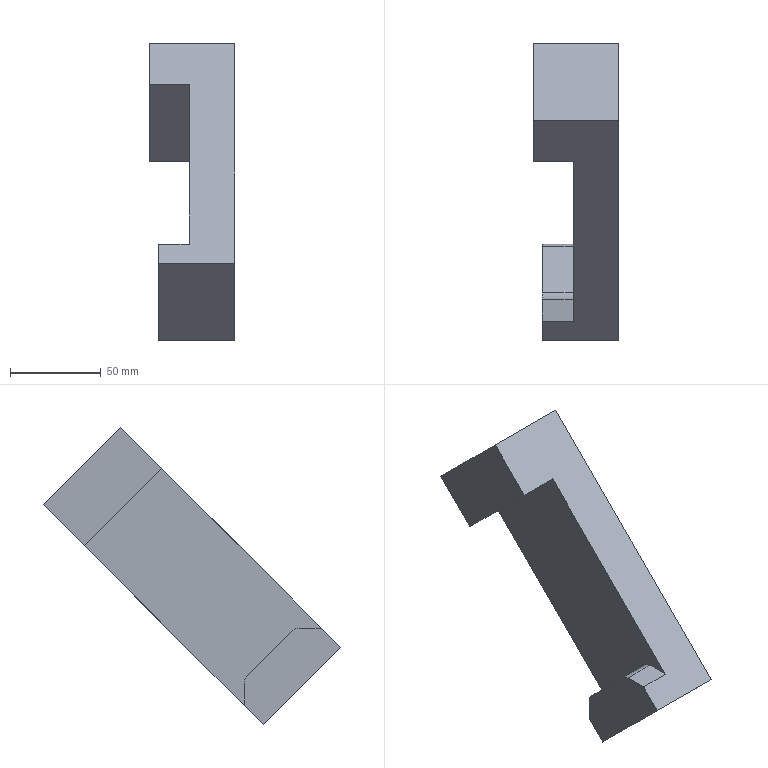Part | NX | features solid 2 | 1 solid | 14 faces | box 47 x 163.342 x 163.342 mm | volume 322522 mm3 | plane 12 | cylinder 2 | commonest cylinder face diameters 10 x2
STEP:
#1=CARTESIAN_POINT('',(757.,887.53,-215.901));
#2=VERTEX_POINT('',#1);
#3=CARTESIAN_POINT('',(757.,975.212,-128.22));
#4=VERTEX_POINT('',#3);
#5=CARTESIAN_POINT('',(757.,937.382,-166.05));
#6=DIRECTION('',(0.,0.7071,0.7071));
#7=VECTOR('',#6,1000.);
#8=LINE('',#5,#7);
#9=EDGE_CURVE('',#2,#4,#8,.T.);
#10=ORIENTED_EDGE('',*,*,#9,.T.);
#11=CARTESIAN_POINT('',(757.,1017.638,-170.646));
#12=VERTEX_POINT('',#11);
#13=CARTESIAN_POINT('',(757.,975.212,-128.22));
#14=DIRECTION('',(0.,0.7071,-0.7071));
#15=VECTOR('',#14,1000.);
#16=LINE('',#13,#15);
#17=EDGE_CURVE('',#4,#12,#16,.T.);
#18=ORIENTED_EDGE('',*,*,#17,.T.);
#19=CARTESIAN_POINT('',(757.,929.957,-258.327));
#20=VERTEX_POINT('',#19);
#21=CARTESIAN_POINT('',(757.,979.808,-208.476));
#22=DIRECTION('',(0.,-0.7071,-0.7071));
#23=VECTOR('',#22,1000.);
#24=LINE('',#21,#23);
#25=EDGE_CURVE('',#12,#20,#24,.T.);
#26=ORIENTED_EDGE('',*,*,#25,.T.);
#27=CARTESIAN_POINT('',(757.,929.957,-246.256));
#28=VERTEX_POINT('',#27);
#29=CARTESIAN_POINT('',(757.,929.957,-258.327));
#30=DIRECTION('',(0.,0.,1.));
#31=VECTOR('',#30,1000.);
#32=LINE('',#29,#31);
#33=EDGE_CURVE('',#28,#20,#32,.F.);
#34=ORIENTED_EDGE('',*,*,#33,.F.);
#35=CARTESIAN_POINT('',(757.,928.492,-242.721));
#36=VERTEX_POINT('',#35);
#37=CARTESIAN_POINT('',(757.,924.957,-246.256));
#38=DIRECTION('',(1.,0.,0.));
#39=DIRECTION('',(0.,-0.9962,-0.08716));
#40=AXIS2_PLACEMENT_3D('',#37,#38,#39);
#41=CIRCLE('',#40,5.);
#42=EDGE_CURVE('',#36,#28,#41,.F.);
#43=ORIENTED_EDGE('',*,*,#42,.F.);
#44=CARTESIAN_POINT('',(757.,903.137,-217.365));
#45=VERTEX_POINT('',#44);
#46=CARTESIAN_POINT('',(757.,894.602,-208.83));
#47=DIRECTION('',(0.,0.7071,-0.7071));
#48=VECTOR('',#47,1000.);
#49=LINE('',#46,#48);
#50=EDGE_CURVE('',#45,#36,#49,.T.);
#51=ORIENTED_EDGE('',*,*,#50,.F.);
#52=CARTESIAN_POINT('',(757.,899.602,-215.901));
#53=VERTEX_POINT('',#52);
#54=CARTESIAN_POINT('',(757.,899.602,-220.901));
#55=DIRECTION('',(1.,0.,0.));
#56=DIRECTION('',(0.,-0.9962,-0.08716));
#57=AXIS2_PLACEMENT_3D('',#54,#55,#56);
#58=CIRCLE('',#57,5.);
#59=EDGE_CURVE('',#53,#45,#58,.F.);
#60=ORIENTED_EDGE('',*,*,#59,.F.);
#61=CARTESIAN_POINT('',(757.,901.673,-215.901));
#62=DIRECTION('',(0.,-1.,0.));
#63=VECTOR('',#62,1000.);
#64=LINE('',#61,#63);
#65=EDGE_CURVE('',#2,#53,#64,.F.);
#66=ORIENTED_EDGE('',*,*,#65,.F.);
#67=EDGE_LOOP('',(#10,#18,#26,#34,#43,#51,#60,#66));
#68=FACE_BOUND('',#67,.T.);
#69=CARTESIAN_POINT('',(757.,958.595,-187.263));
#70=DIRECTION('',(-1.,0.,0.));
#71=DIRECTION('',(0.,-0.7071,-0.7071));
#72=AXIS2_PLACEMENT_3D('',#69,#70,#71);
#73=PLANE('',#72);
#74=ADVANCED_FACE('',(#68),#73,.T.);
#75=CARTESIAN_POINT('',(740.,876.924,-226.508));
#76=VERTEX_POINT('',#75);
#77=CARTESIAN_POINT('',(740.,887.53,-215.901));
#78=VERTEX_POINT('',#77);
#79=CARTESIAN_POINT('',(740.,876.924,-226.508));
#80=DIRECTION('',(0.,0.7071,0.7071));
#81=VECTOR('',#80,1000.);
#82=LINE('',#79,#81);
#83=EDGE_CURVE('',#76,#78,#82,.T.);
#84=ORIENTED_EDGE('',*,*,#83,.F.);
#85=CARTESIAN_POINT('',(782.,876.924,-226.508));
#86=VERTEX_POINT('',#85);
#87=CARTESIAN_POINT('',(782.,876.924,-226.508));
#88=DIRECTION('',(-1.,0.,0.));
#89=VECTOR('',#88,1000.);
#90=LINE('',#87,#89);
#91=EDGE_CURVE('',#86,#76,#90,.T.);
#92=ORIENTED_EDGE('',*,*,#91,.F.);
#93=CARTESIAN_POINT('',(782.,997.839,-105.592));
#94=VERTEX_POINT('',#93);
#95=CARTESIAN_POINT('',(782.,937.382,-166.05));
#96=DIRECTION('',(0.,-0.7071,-0.7071));
#97=VECTOR('',#96,1000.);
#98=LINE('',#95,#97);
#99=EDGE_CURVE('',#94,#86,#98,.T.);
#100=ORIENTED_EDGE('',*,*,#99,.F.);
#101=CARTESIAN_POINT('',(735.,997.839,-105.592));
#102=VERTEX_POINT('',#101);
#103=CARTESIAN_POINT('',(782.,997.839,-105.592));
#104=DIRECTION('',(-1.,0.,0.));
#105=VECTOR('',#104,1000.);
#106=LINE('',#103,#105);
#107=EDGE_CURVE('',#94,#102,#106,.T.);
#108=ORIENTED_EDGE('',*,*,#107,.T.);
#109=CARTESIAN_POINT('',(735.,975.212,-128.22));
#110=VERTEX_POINT('',#109);
#111=CARTESIAN_POINT('',(735.,997.839,-105.592));
#112=DIRECTION('',(0.,-0.7071,-0.7071));
#113=VECTOR('',#112,1000.);
#114=LINE('',#111,#113);
#115=EDGE_CURVE('',#110,#102,#114,.F.);
#116=ORIENTED_EDGE('',*,*,#115,.F.);
#117=CARTESIAN_POINT('',(757.,975.212,-128.22));
#118=DIRECTION('',(1.,0.,0.));
#119=VECTOR('',#118,1000.);
#120=LINE('',#117,#119);
#121=EDGE_CURVE('',#4,#110,#120,.F.);
#122=ORIENTED_EDGE('',*,*,#121,.F.);
#123=ORIENTED_EDGE('',*,*,#9,.F.);
#124=CARTESIAN_POINT('',(782.,887.53,-215.901));
#125=DIRECTION('',(1.,0.,0.));
#126=VECTOR('',#125,1000.);
#127=LINE('',#124,#126);
#128=EDGE_CURVE('',#78,#2,#127,.T.);
#129=ORIENTED_EDGE('',*,*,#128,.F.);
#130=EDGE_LOOP('',(#84,#92,#100,#108,#116,#122,#123,#129));
#131=FACE_BOUND('',#130,.T.);
#132=CARTESIAN_POINT('',(782.,937.382,-166.05));
#133=DIRECTION('',(0.,-0.7071,0.7071));
#134=DIRECTION('',(1.,0.,0.));
#135=AXIS2_PLACEMENT_3D('',#132,#133,#134);
#136=PLANE('',#135);
#137=ADVANCED_FACE('',(#131),#136,.T.);
#138=ORIENTED_EDGE('',*,*,#107,.F.);
#139=CARTESIAN_POINT('',(782.,1040.266,-148.019));
#140=VERTEX_POINT('',#139);
#141=CARTESIAN_POINT('',(782.,1019.052,-126.806));
#142=DIRECTION('',(0.,-0.7071,0.7071));
#143=VECTOR('',#142,1000.);
#144=LINE('',#141,#143);
#145=EDGE_CURVE('',#140,#94,#144,.T.);
#146=ORIENTED_EDGE('',*,*,#145,.F.);
#147=CARTESIAN_POINT('',(735.,1040.266,-148.019));
#148=VERTEX_POINT('',#147);
#149=CARTESIAN_POINT('',(782.,1040.266,-148.019));
#150=DIRECTION('',(-1.,0.,0.));
#151=VECTOR('',#150,1000.);
#152=LINE('',#149,#151);
#153=EDGE_CURVE('',#140,#148,#152,.T.);
#154=ORIENTED_EDGE('',*,*,#153,.T.);
#155=CARTESIAN_POINT('',(735.,997.839,-105.592));
#156=DIRECTION('',(0.,0.7071,-0.7071));
#157=VECTOR('',#156,1000.);
#158=LINE('',#155,#157);
#159=EDGE_CURVE('',#102,#148,#158,.T.);
#160=ORIENTED_EDGE('',*,*,#159,.F.);
#161=EDGE_LOOP('',(#138,#146,#154,#160));
#162=FACE_BOUND('',#161,.T.);
#163=CARTESIAN_POINT('',(782.,1019.052,-126.806));
#164=DIRECTION('',(0.,0.7071,0.7071));
#165=DIRECTION('',(-1.,0.,0.));
#166=AXIS2_PLACEMENT_3D('',#163,#164,#165);
#167=PLANE('',#166);
#168=ADVANCED_FACE('',(#162),#167,.T.);
#169=ORIENTED_EDGE('',*,*,#25,.F.);
#170=CARTESIAN_POINT('',(735.,1017.638,-170.646));
#171=VERTEX_POINT('',#170);
#172=CARTESIAN_POINT('',(757.,1017.638,-170.646));
#173=DIRECTION('',(1.,0.,0.));
#174=VECTOR('',#173,1000.);
#175=LINE('',#172,#174);
#176=EDGE_CURVE('',#12,#171,#175,.F.);
#177=ORIENTED_EDGE('',*,*,#176,.T.);
#178=CARTESIAN_POINT('',(735.,1040.266,-148.019));
#179=DIRECTION('',(0.,-0.7071,-0.7071));
#180=VECTOR('',#179,1000.);
#181=LINE('',#178,#180);
#182=EDGE_CURVE('',#171,#148,#181,.F.);
#183=ORIENTED_EDGE('',*,*,#182,.T.);
#184=ORIENTED_EDGE('',*,*,#153,.F.);
#185=CARTESIAN_POINT('',(782.,919.35,-268.934));
#186=VERTEX_POINT('',#185);
#187=CARTESIAN_POINT('',(782.,979.808,-208.476));
#188=DIRECTION('',(0.,0.7071,0.7071));
#189=VECTOR('',#188,1000.);
#190=LINE('',#187,#189);
#191=EDGE_CURVE('',#186,#140,#190,.T.);
#192=ORIENTED_EDGE('',*,*,#191,.F.);
#193=CARTESIAN_POINT('',(740.,919.35,-268.934));
#194=VERTEX_POINT('',#193);
#195=CARTESIAN_POINT('',(782.,919.35,-268.934));
#196=DIRECTION('',(-1.,0.,0.));
#197=VECTOR('',#196,1000.);
#198=LINE('',#195,#197);
#199=EDGE_CURVE('',#186,#194,#198,.T.);
#200=ORIENTED_EDGE('',*,*,#199,.T.);
#201=CARTESIAN_POINT('',(740.,929.957,-258.327));
#202=VERTEX_POINT('',#201);
#203=CARTESIAN_POINT('',(740.,919.35,-268.934));
#204=DIRECTION('',(0.,0.7071,0.7071));
#205=VECTOR('',#204,1000.);
#206=LINE('',#203,#205);
#207=EDGE_CURVE('',#194,#202,#206,.T.);
#208=ORIENTED_EDGE('',*,*,#207,.T.);
#209=CARTESIAN_POINT('',(782.,929.957,-258.327));
#210=DIRECTION('',(-1.,0.,0.));
#211=VECTOR('',#210,1000.);
#212=LINE('',#209,#211);
#213=EDGE_CURVE('',#20,#202,#212,.T.);
#214=ORIENTED_EDGE('',*,*,#213,.F.);
#215=EDGE_LOOP('',(#169,#177,#183,#184,#192,#200,#208,#214));
#216=FACE_BOUND('',#215,.T.);
#217=CARTESIAN_POINT('',(782.,979.808,-208.476));
#218=DIRECTION('',(0.,0.7071,-0.7071));
#219=DIRECTION('',(-1.,0.,0.));
#220=AXIS2_PLACEMENT_3D('',#217,#218,#219);
#221=PLANE('',#220);
#222=ADVANCED_FACE('',(#216),#221,.T.);
#223=CARTESIAN_POINT('',(782.,898.137,-247.721));
#224=DIRECTION('',(0.,0.7071,-0.7071));
#225=VECTOR('',#224,1000.);
#226=LINE('',#223,#225);
#227=EDGE_CURVE('',#86,#186,#226,.T.);
#228=ORIENTED_EDGE('',*,*,#227,.T.);
#229=ORIENTED_EDGE('',*,*,#191,.T.);
#230=ORIENTED_EDGE('',*,*,#145,.T.);
#231=ORIENTED_EDGE('',*,*,#99,.T.);
#232=EDGE_LOOP('',(#228,#229,#230,#231));
#233=FACE_BOUND('',#232,.T.);
#234=CARTESIAN_POINT('',(782.,958.595,-187.263));
#235=DIRECTION('',(1.,0.,0.));
#236=DIRECTION('',(0.,0.7071,0.7071));
#237=AXIS2_PLACEMENT_3D('',#234,#235,#236);
#238=PLANE('',#237);
#239=ADVANCED_FACE('',(#233),#238,.T.);
#240=ORIENTED_EDGE('',*,*,#227,.F.);
#241=ORIENTED_EDGE('',*,*,#91,.T.);
#242=CARTESIAN_POINT('',(740.,876.924,-226.508));
#243=DIRECTION('',(0.,0.7071,-0.7071));
#244=VECTOR('',#243,1000.);
#245=LINE('',#242,#244);
#246=EDGE_CURVE('',#76,#194,#245,.T.);
#247=ORIENTED_EDGE('',*,*,#246,.T.);
#248=ORIENTED_EDGE('',*,*,#199,.F.);
#249=EDGE_LOOP('',(#240,#241,#247,#248));
#250=FACE_BOUND('',#249,.T.);
#251=CARTESIAN_POINT('',(782.,898.137,-247.721));
#252=DIRECTION('',(0.,-0.7071,-0.7071));
#253=DIRECTION('',(1.,0.,0.));
#254=AXIS2_PLACEMENT_3D('',#251,#252,#253);
#255=PLANE('',#254);
#256=ADVANCED_FACE('',(#250),#255,.T.);
#257=ORIENTED_EDGE('',*,*,#182,.F.);
#258=CARTESIAN_POINT('',(735.,975.212,-128.22));
#259=DIRECTION('',(0.,0.7071,-0.7071));
#260=VECTOR('',#259,1000.);
#261=LINE('',#258,#260);
#262=EDGE_CURVE('',#110,#171,#261,.T.);
#263=ORIENTED_EDGE('',*,*,#262,.F.);
#264=ORIENTED_EDGE('',*,*,#115,.T.);
#265=ORIENTED_EDGE('',*,*,#159,.T.);
#266=EDGE_LOOP('',(#257,#263,#264,#265));
#267=FACE_BOUND('',#266,.T.);
#268=CARTESIAN_POINT('',(735.,997.839,-105.592));
#269=DIRECTION('',(1.,0.,0.));
#270=DIRECTION('',(0.,0.7071,-0.7071));
#271=AXIS2_PLACEMENT_3D('',#268,#269,#270);
#272=PLANE('',#271);
#273=ADVANCED_FACE('',(#267),#272,.F.);
#274=ORIENTED_EDGE('',*,*,#262,.T.);
#275=ORIENTED_EDGE('',*,*,#176,.F.);
#276=ORIENTED_EDGE('',*,*,#17,.F.);
#277=ORIENTED_EDGE('',*,*,#121,.T.);
#278=EDGE_LOOP('',(#274,#275,#276,#277));
#279=FACE_BOUND('',#278,.T.);
#280=CARTESIAN_POINT('',(757.,975.212,-128.22));
#281=DIRECTION('',(0.,-0.7071,-0.7071));
#282=DIRECTION('',(1.,0.,0.));
#283=AXIS2_PLACEMENT_3D('',#280,#281,#282);
#284=PLANE('',#283);
#285=ADVANCED_FACE('',(#279),#284,.T.);
#286=ORIENTED_EDGE('',*,*,#50,.T.);
#287=CARTESIAN_POINT('',(740.,928.492,-242.721));
#288=VERTEX_POINT('',#287);
#289=CARTESIAN_POINT('',(757.,928.492,-242.721));
#290=DIRECTION('',(-1.,0.,0.));
#291=VECTOR('',#290,1000.);
#292=LINE('',#289,#291);
#293=EDGE_CURVE('',#288,#36,#292,.F.);
#294=ORIENTED_EDGE('',*,*,#293,.F.);
#295=CARTESIAN_POINT('',(740.,903.137,-217.365));
#296=VERTEX_POINT('',#295);
#297=CARTESIAN_POINT('',(740.,894.602,-208.83));
#298=DIRECTION('',(0.,0.7071,-0.7071));
#299=VECTOR('',#298,1000.);
#300=LINE('',#297,#299);
#301=EDGE_CURVE('',#296,#288,#300,.T.);
#302=ORIENTED_EDGE('',*,*,#301,.F.);
#303=CARTESIAN_POINT('',(757.,903.137,-217.365));
#304=DIRECTION('',(1.,0.,0.));
#305=VECTOR('',#304,1000.);
#306=LINE('',#303,#305);
#307=EDGE_CURVE('',#45,#296,#306,.F.);
#308=ORIENTED_EDGE('',*,*,#307,.F.);
#309=EDGE_LOOP('',(#286,#294,#302,#308));
#310=FACE_BOUND('',#309,.T.);
#311=CARTESIAN_POINT('',(757.,894.602,-208.83));
#312=DIRECTION('',(0.,0.7071,0.7071));
#313=DIRECTION('',(-1.,0.,0.));
#314=AXIS2_PLACEMENT_3D('',#311,#312,#313);
#315=PLANE('',#314);
#316=ADVANCED_FACE('',(#310),#315,.T.);
#317=ORIENTED_EDGE('',*,*,#301,.T.);
#318=CARTESIAN_POINT('',(740.,929.957,-246.256));
#319=VERTEX_POINT('',#318);
#320=CARTESIAN_POINT('',(740.,924.957,-246.256));
#321=DIRECTION('',(1.,0.,0.));
#322=DIRECTION('',(0.,-0.9962,-0.08716));
#323=AXIS2_PLACEMENT_3D('',#320,#321,#322);
#324=CIRCLE('',#323,5.);
#325=EDGE_CURVE('',#319,#288,#324,.T.);
#326=ORIENTED_EDGE('',*,*,#325,.F.);
#327=CARTESIAN_POINT('',(740.,929.957,-226.508));
#328=DIRECTION('',(0.,0.,-1.));
#329=VECTOR('',#328,1000.);
#330=LINE('',#327,#329);
#331=EDGE_CURVE('',#202,#319,#330,.F.);
#332=ORIENTED_EDGE('',*,*,#331,.F.);
#333=ORIENTED_EDGE('',*,*,#207,.F.);
#334=ORIENTED_EDGE('',*,*,#246,.F.);
#335=ORIENTED_EDGE('',*,*,#83,.T.);
#336=CARTESIAN_POINT('',(740.,899.602,-215.901));
#337=VERTEX_POINT('',#336);
#338=CARTESIAN_POINT('',(740.,876.924,-215.901));
#339=DIRECTION('',(0.,1.,0.));
#340=VECTOR('',#339,1000.);
#341=LINE('',#338,#340);
#342=EDGE_CURVE('',#337,#78,#341,.F.);
#343=ORIENTED_EDGE('',*,*,#342,.F.);
#344=CARTESIAN_POINT('',(740.,899.602,-220.901));
#345=DIRECTION('',(1.,0.,0.));
#346=DIRECTION('',(0.,-0.9962,-0.08716));
#347=AXIS2_PLACEMENT_3D('',#344,#345,#346);
#348=CIRCLE('',#347,5.);
#349=EDGE_CURVE('',#296,#337,#348,.T.);
#350=ORIENTED_EDGE('',*,*,#349,.F.);
#351=EDGE_LOOP('',(#317,#326,#332,#333,#334,#335,#343,#350));
#352=FACE_BOUND('',#351,.T.);
#353=CARTESIAN_POINT('',(740.,876.924,-226.508));
#354=DIRECTION('',(-1.,0.,0.));
#355=DIRECTION('',(0.,-0.7071,-0.7071));
#356=AXIS2_PLACEMENT_3D('',#353,#354,#355);
#357=PLANE('',#356);
#358=ADVANCED_FACE('',(#352),#357,.T.);
#359=ORIENTED_EDGE('',*,*,#342,.T.);
#360=ORIENTED_EDGE('',*,*,#128,.T.);
#361=ORIENTED_EDGE('',*,*,#65,.T.);
#362=CARTESIAN_POINT('',(757.,899.602,-215.901));
#363=DIRECTION('',(-1.,0.,0.));
#364=VECTOR('',#363,1000.);
#365=LINE('',#362,#364);
#366=EDGE_CURVE('',#337,#53,#365,.F.);
#367=ORIENTED_EDGE('',*,*,#366,.F.);
#368=EDGE_LOOP('',(#359,#360,#361,#367));
#369=FACE_BOUND('',#368,.T.);
#370=CARTESIAN_POINT('',(757.,901.673,-215.901));
#371=DIRECTION('',(0.,0.,-1.));
#372=DIRECTION('',(0.,1.,0.));
#373=AXIS2_PLACEMENT_3D('',#370,#371,#372);
#374=PLANE('',#373);
#375=ADVANCED_FACE('',(#369),#374,.F.);
#376=ORIENTED_EDGE('',*,*,#33,.T.);
#377=ORIENTED_EDGE('',*,*,#213,.T.);
#378=ORIENTED_EDGE('',*,*,#331,.T.);
#379=CARTESIAN_POINT('',(782.,929.957,-246.256));
#380=DIRECTION('',(1.,0.,0.));
#381=VECTOR('',#380,1000.);
#382=LINE('',#379,#381);
#383=EDGE_CURVE('',#28,#319,#382,.F.);
#384=ORIENTED_EDGE('',*,*,#383,.F.);
#385=EDGE_LOOP('',(#376,#377,#378,#384));
#386=FACE_BOUND('',#385,.T.);
#387=CARTESIAN_POINT('',(782.,929.957,-258.327));
#388=DIRECTION('',(0.,-1.,0.));
#389=DIRECTION('',(0.,0.,-1.));
#390=AXIS2_PLACEMENT_3D('',#387,#388,#389);
#391=PLANE('',#390);
#392=ADVANCED_FACE('',(#386),#391,.F.);
#393=ORIENTED_EDGE('',*,*,#59,.T.);
#394=ORIENTED_EDGE('',*,*,#307,.T.);
#395=ORIENTED_EDGE('',*,*,#349,.T.);
#396=ORIENTED_EDGE('',*,*,#366,.T.);
#397=EDGE_LOOP('',(#393,#394,#395,#396));
#398=FACE_BOUND('',#397,.T.);
#399=CARTESIAN_POINT('',(757.,899.602,-220.901));
#400=DIRECTION('',(1.,0.,0.));
#401=DIRECTION('',(0.,0.9962,0.08716));
#402=AXIS2_PLACEMENT_3D('',#399,#400,#401);
#403=CYLINDRICAL_SURFACE('',#402,5.);
#404=ADVANCED_FACE('',(#398),#403,.T.);
#405=ORIENTED_EDGE('',*,*,#325,.T.);
#406=ORIENTED_EDGE('',*,*,#293,.T.);
#407=ORIENTED_EDGE('',*,*,#42,.T.);
#408=ORIENTED_EDGE('',*,*,#383,.T.);
#409=EDGE_LOOP('',(#405,#406,#407,#408));
#410=FACE_BOUND('',#409,.T.);
#411=CARTESIAN_POINT('',(757.,924.957,-246.256));
#412=DIRECTION('',(-1.,0.,0.));
#413=DIRECTION('',(0.,-0.9962,-0.08716));
#414=AXIS2_PLACEMENT_3D('',#411,#412,#413);
#415=CYLINDRICAL_SURFACE('',#414,5.);
#416=ADVANCED_FACE('',(#410),#415,.T.);
#417=CLOSED_SHELL('',(#74,#137,#168,#222,#239,#256,#273,#285,#316,#358,#375,#392,#404,#416));
#418=MANIFOLD_SOLID_BREP('',#417);
#419=(LENGTH_UNIT()NAMED_UNIT(*)SI_UNIT(.MILLI.,.METRE.));
#420=UNCERTAINTY_MEASURE_WITH_UNIT(LENGTH_MEASURE(0.00001),#419,'','');
#421=(NAMED_UNIT(*)PLANE_ANGLE_UNIT()SI_UNIT($,.RADIAN.));
#422=(NAMED_UNIT(*)SI_UNIT($,.STERADIAN.)SOLID_ANGLE_UNIT());
#423=(GEOMETRIC_REPRESENTATION_CONTEXT(3)GLOBAL_UNCERTAINTY_ASSIGNED_CONTEXT((#420))GLOBAL_UNIT_ASSIGNED_CONTEXT((#419,#421,#422))REPRESENTATION_CONTEXT('',''));
#424=ADVANCED_BREP_SHAPE_REPRESENTATION('',(#418),#423);